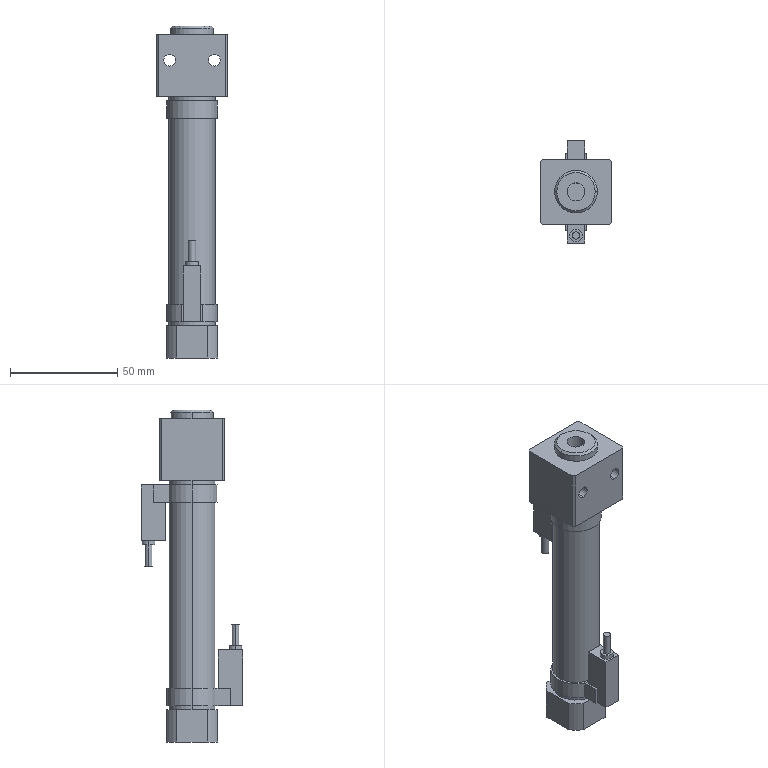Part | NX | features BREP 1 | 1 solid | 102 faces | box 33.5 x 47.6 x 155 mm | volume 76841 mm3 | plane 54 | cylinder 42 | cone 6 | commonest cylinder face diameters 23.6 x8 21.6 x6 3.4 x4 5.5 x4 6 x4 8.57 x4